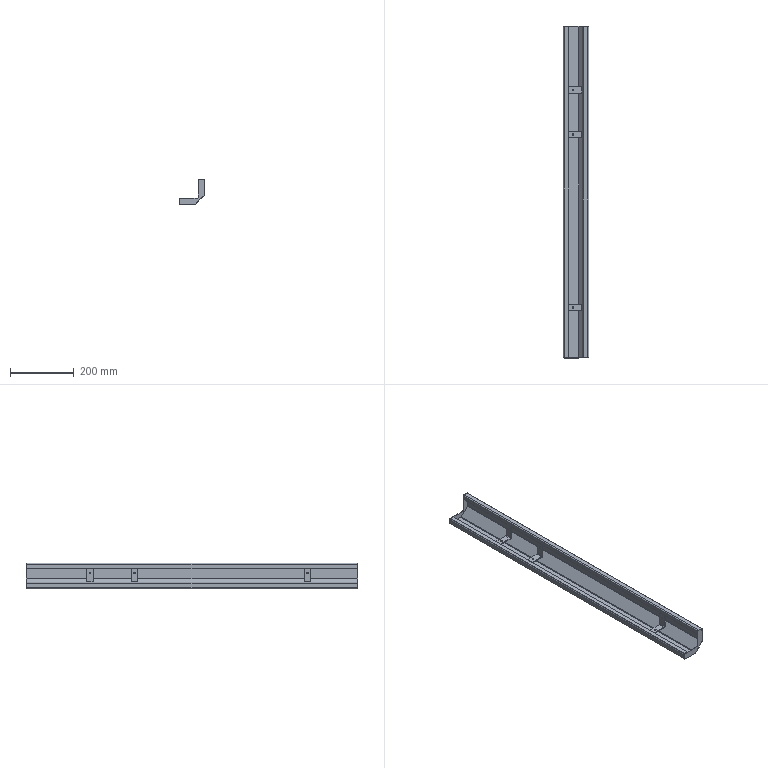Part | SolidWorks | features FlatPattern 4, EdgeFlange 2, HoleWzd 2, LPattern 2, SMBaseFlange 2, SheetMetal 2, Fillet 1, ICE 1, MirrorSolid 1 | 6 solids | 140 faces | box 80 x 1039 x 80 mm | volume 334294 mm3 | plane 96 | cylinder 44 | commonest cylinder face diameters 7 x18 5 x12 4 x9 10 x3 8 x2